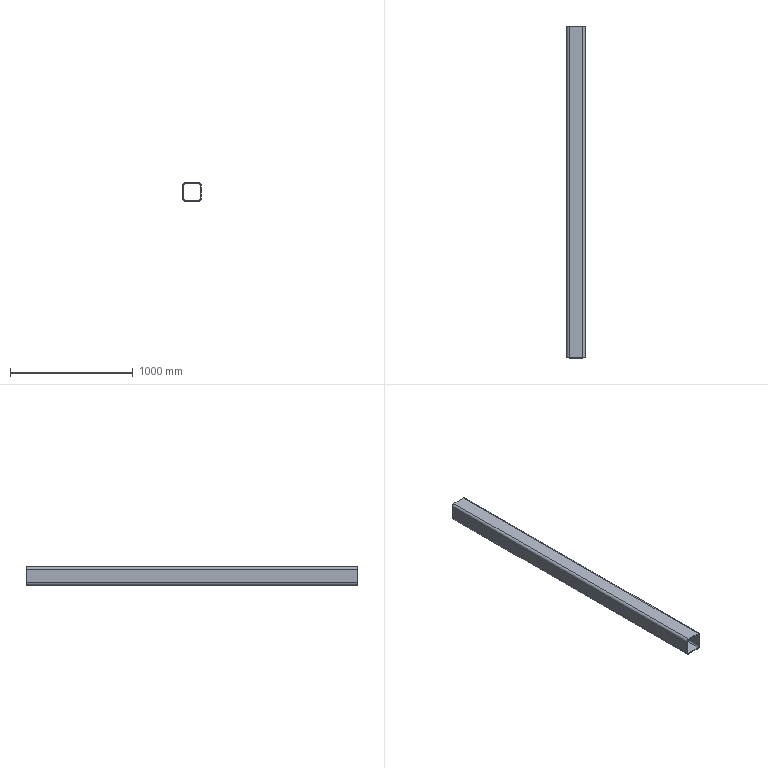Part | SolidWorks | features ICE 2, Extrusion 1, LPattern 1 | 1 solid | 210 faces | box 150 x 2710 x 150 mm | volume 11443018 mm3 | cylinder 188 | plane 22 | commonest cylinder face diameters 5.2 x180 24 x4 40 x4